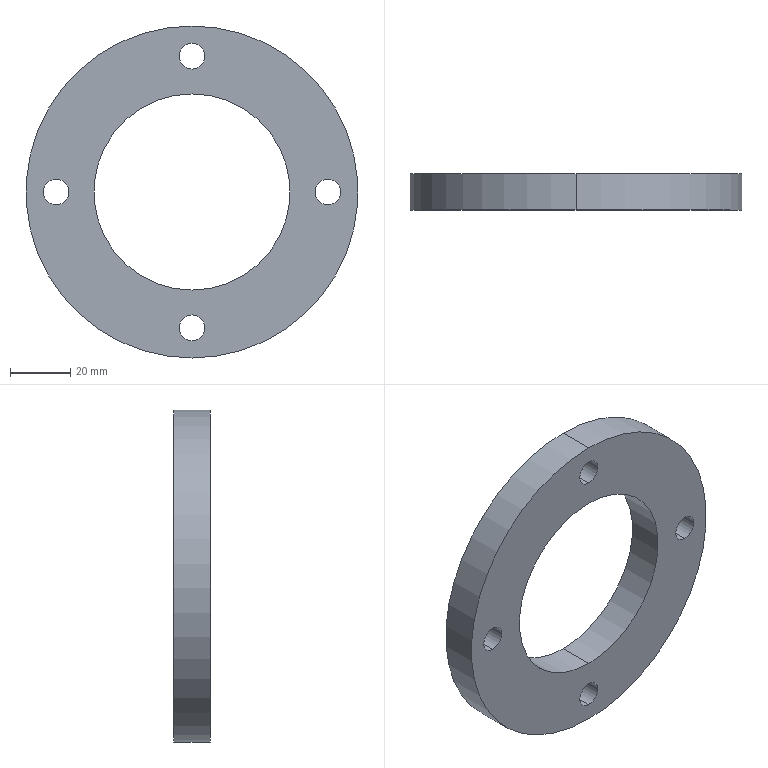Part | SolidWorks | features BaseBody 1 | 1 solid | 14 faces | box 110 x 12 x 110 mm | volume 71496 mm3 | cylinder 12 | plane 2 | commonest cylinder face diameters 8.5 x8 65 x2 110 x2
STEP:
#1=CARTESIAN_POINT('',(0.,12.,32.5));
#2=VERTEX_POINT('',#1);
#3=CARTESIAN_POINT('',(0.,12.,-32.5));
#4=VERTEX_POINT('',#3);
#5=CARTESIAN_POINT('',(0.,12.,0.));
#6=DIRECTION('',(0.,-1.,0.));
#7=DIRECTION('',(0.,0.,-1.));
#8=AXIS2_PLACEMENT_3D('',#5,#6,#7);
#9=CIRCLE('',#8,32.5);
#10=EDGE_CURVE('',#2,#4,#9,.T.);
#11=ORIENTED_EDGE('',*,*,#10,.F.);
#12=CARTESIAN_POINT('',(0.,0.,32.5));
#13=VERTEX_POINT('',#12);
#14=CARTESIAN_POINT('',(0.,12.,32.5));
#15=DIRECTION('',(0.,-1.,0.));
#16=VECTOR('',#15,1000.);
#17=LINE('',#14,#16);
#18=EDGE_CURVE('',#2,#13,#17,.T.);
#19=ORIENTED_EDGE('',*,*,#18,.T.);
#20=CARTESIAN_POINT('',(0.,0.,-32.5));
#21=VERTEX_POINT('',#20);
#22=CARTESIAN_POINT('',(0.,0.,0.));
#23=DIRECTION('',(0.,1.,0.));
#24=DIRECTION('',(0.,0.,-1.));
#25=AXIS2_PLACEMENT_3D('',#22,#23,#24);
#26=CIRCLE('',#25,32.5);
#27=EDGE_CURVE('',#21,#13,#26,.T.);
#28=ORIENTED_EDGE('',*,*,#27,.F.);
#29=CARTESIAN_POINT('',(0.,12.,-32.5));
#30=DIRECTION('',(0.,-1.,0.));
#31=VECTOR('',#30,1000.);
#32=LINE('',#29,#31);
#33=EDGE_CURVE('',#4,#21,#32,.T.);
#34=ORIENTED_EDGE('',*,*,#33,.F.);
#35=EDGE_LOOP('',(#11,#19,#28,#34));
#36=FACE_OUTER_BOUND('',#35,.T.);
#37=CARTESIAN_POINT('',(0.,12.,0.));
#38=DIRECTION('',(0.,-1.,0.));
#39=DIRECTION('',(0.,0.,-1.));
#40=AXIS2_PLACEMENT_3D('',#37,#38,#39);
#41=CYLINDRICAL_SURFACE('',#40,32.5);
#42=ADVANCED_FACE('',(#36),#41,.F.);
#43=CARTESIAN_POINT('',(0.,12.,55.));
#44=VERTEX_POINT('',#43);
#45=CARTESIAN_POINT('',(0.,12.,-55.));
#46=VERTEX_POINT('',#45);
#47=CARTESIAN_POINT('',(0.,12.,0.));
#48=DIRECTION('',(0.,1.,0.));
#49=DIRECTION('',(0.,0.,-1.));
#50=AXIS2_PLACEMENT_3D('',#47,#48,#49);
#51=CIRCLE('',#50,55.);
#52=EDGE_CURVE('',#44,#46,#51,.T.);
#53=ORIENTED_EDGE('',*,*,#52,.F.);
#54=CARTESIAN_POINT('',(0.,0.,55.));
#55=VERTEX_POINT('',#54);
#56=CARTESIAN_POINT('',(0.,12.,55.));
#57=DIRECTION('',(0.,-1.,0.));
#58=VECTOR('',#57,1000.);
#59=LINE('',#56,#58);
#60=EDGE_CURVE('',#44,#55,#59,.T.);
#61=ORIENTED_EDGE('',*,*,#60,.T.);
#62=CARTESIAN_POINT('',(0.,0.,-55.));
#63=VERTEX_POINT('',#62);
#64=CARTESIAN_POINT('',(0.,0.,0.));
#65=DIRECTION('',(0.,1.,0.));
#66=DIRECTION('',(0.,0.,-1.));
#67=AXIS2_PLACEMENT_3D('',#64,#65,#66);
#68=CIRCLE('',#67,55.);
#69=EDGE_CURVE('',#55,#63,#68,.T.);
#70=ORIENTED_EDGE('',*,*,#69,.T.);
#71=CARTESIAN_POINT('',(0.,12.,-55.));
#72=DIRECTION('',(0.,-1.,0.));
#73=VECTOR('',#72,1000.);
#74=LINE('',#71,#73);
#75=EDGE_CURVE('',#46,#63,#74,.T.);
#76=ORIENTED_EDGE('',*,*,#75,.F.);
#77=EDGE_LOOP('',(#53,#61,#70,#76));
#78=FACE_OUTER_BOUND('',#77,.T.);
#79=CARTESIAN_POINT('',(0.,12.,0.));
#80=DIRECTION('',(0.,-1.,0.));
#81=DIRECTION('',(0.,0.,-1.));
#82=AXIS2_PLACEMENT_3D('',#79,#80,#81);
#83=CYLINDRICAL_SURFACE('',#82,55.);
#84=ADVANCED_FACE('',(#78),#83,.T.);
#85=CARTESIAN_POINT('',(0.,0.,-49.25));
#86=VERTEX_POINT('',#85);
#87=CARTESIAN_POINT('',(0.,0.,-40.75));
#88=VERTEX_POINT('',#87);
#89=CARTESIAN_POINT('',(0.,0.,-45.));
#90=DIRECTION('',(0.,1.,0.));
#91=DIRECTION('',(0.,0.,1.));
#92=AXIS2_PLACEMENT_3D('',#89,#90,#91);
#93=CIRCLE('',#92,4.25);
#94=EDGE_CURVE('',#86,#88,#93,.T.);
#95=ORIENTED_EDGE('',*,*,#94,.F.);
#96=CARTESIAN_POINT('',(0.,12.,-49.25));
#97=VERTEX_POINT('',#96);
#98=CARTESIAN_POINT('',(0.,12.,-49.25));
#99=DIRECTION('',(0.,1.,0.));
#100=VECTOR('',#99,1000.);
#101=LINE('',#98,#100);
#102=EDGE_CURVE('',#86,#97,#101,.T.);
#103=ORIENTED_EDGE('',*,*,#102,.T.);
#104=CARTESIAN_POINT('',(0.,12.,-40.75));
#105=VERTEX_POINT('',#104);
#106=CARTESIAN_POINT('',(0.,12.,-45.));
#107=DIRECTION('',(0.,-1.,0.));
#108=DIRECTION('',(0.,0.,1.));
#109=AXIS2_PLACEMENT_3D('',#106,#107,#108);
#110=CIRCLE('',#109,4.25);
#111=EDGE_CURVE('',#105,#97,#110,.T.);
#112=ORIENTED_EDGE('',*,*,#111,.F.);
#113=CARTESIAN_POINT('',(0.,12.,-40.75));
#114=DIRECTION('',(0.,1.,0.));
#115=VECTOR('',#114,1000.);
#116=LINE('',#113,#115);
#117=EDGE_CURVE('',#88,#105,#116,.T.);
#118=ORIENTED_EDGE('',*,*,#117,.F.);
#119=EDGE_LOOP('',(#95,#103,#112,#118));
#120=FACE_OUTER_BOUND('',#119,.T.);
#121=CARTESIAN_POINT('',(0.,12.,-45.));
#122=DIRECTION('',(0.,1.,0.));
#123=DIRECTION('',(0.,0.,1.));
#124=AXIS2_PLACEMENT_3D('',#121,#122,#123);
#125=CYLINDRICAL_SURFACE('',#124,4.25);
#126=ADVANCED_FACE('',(#120),#125,.F.);
#127=CARTESIAN_POINT('',(-45.,0.,-4.25));
#128=VERTEX_POINT('',#127);
#129=CARTESIAN_POINT('',(-45.,0.,4.25));
#130=VERTEX_POINT('',#129);
#131=CARTESIAN_POINT('',(-45.,0.,0.));
#132=DIRECTION('',(0.,1.,0.));
#133=DIRECTION('',(0.,0.,1.));
#134=AXIS2_PLACEMENT_3D('',#131,#132,#133);
#135=CIRCLE('',#134,4.25);
#136=EDGE_CURVE('',#128,#130,#135,.T.);
#137=ORIENTED_EDGE('',*,*,#136,.F.);
#138=CARTESIAN_POINT('',(-45.,12.,-4.25));
#139=VERTEX_POINT('',#138);
#140=CARTESIAN_POINT('',(-45.,12.,-4.25));
#141=DIRECTION('',(0.,1.,0.));
#142=VECTOR('',#141,1000.);
#143=LINE('',#140,#142);
#144=EDGE_CURVE('',#128,#139,#143,.T.);
#145=ORIENTED_EDGE('',*,*,#144,.T.);
#146=CARTESIAN_POINT('',(-45.,12.,4.25));
#147=VERTEX_POINT('',#146);
#148=CARTESIAN_POINT('',(-45.,12.,0.));
#149=DIRECTION('',(0.,-1.,0.));
#150=DIRECTION('',(0.,0.,1.));
#151=AXIS2_PLACEMENT_3D('',#148,#149,#150);
#152=CIRCLE('',#151,4.25);
#153=EDGE_CURVE('',#147,#139,#152,.T.);
#154=ORIENTED_EDGE('',*,*,#153,.F.);
#155=CARTESIAN_POINT('',(-45.,12.,4.25));
#156=DIRECTION('',(0.,1.,0.));
#157=VECTOR('',#156,1000.);
#158=LINE('',#155,#157);
#159=EDGE_CURVE('',#130,#147,#158,.T.);
#160=ORIENTED_EDGE('',*,*,#159,.F.);
#161=EDGE_LOOP('',(#137,#145,#154,#160));
#162=FACE_OUTER_BOUND('',#161,.T.);
#163=CARTESIAN_POINT('',(-45.,12.,0.));
#164=DIRECTION('',(0.,1.,0.));
#165=DIRECTION('',(0.,0.,1.));
#166=AXIS2_PLACEMENT_3D('',#163,#164,#165);
#167=CYLINDRICAL_SURFACE('',#166,4.25);
#168=ADVANCED_FACE('',(#162),#167,.F.);
#169=CARTESIAN_POINT('',(0.,0.,40.75));
#170=VERTEX_POINT('',#169);
#171=CARTESIAN_POINT('',(0.,0.,49.25));
#172=VERTEX_POINT('',#171);
#173=CARTESIAN_POINT('',(0.,0.,45.));
#174=DIRECTION('',(0.,1.,0.));
#175=DIRECTION('',(0.,0.,1.));
#176=AXIS2_PLACEMENT_3D('',#173,#174,#175);
#177=CIRCLE('',#176,4.25);
#178=EDGE_CURVE('',#170,#172,#177,.T.);
#179=ORIENTED_EDGE('',*,*,#178,.F.);
#180=CARTESIAN_POINT('',(0.,12.,40.75));
#181=VERTEX_POINT('',#180);
#182=CARTESIAN_POINT('',(0.,12.,40.75));
#183=DIRECTION('',(0.,1.,0.));
#184=VECTOR('',#183,1000.);
#185=LINE('',#182,#184);
#186=EDGE_CURVE('',#170,#181,#185,.T.);
#187=ORIENTED_EDGE('',*,*,#186,.T.);
#188=CARTESIAN_POINT('',(0.,12.,49.25));
#189=VERTEX_POINT('',#188);
#190=CARTESIAN_POINT('',(0.,12.,45.));
#191=DIRECTION('',(0.,-1.,0.));
#192=DIRECTION('',(0.,0.,1.));
#193=AXIS2_PLACEMENT_3D('',#190,#191,#192);
#194=CIRCLE('',#193,4.25);
#195=EDGE_CURVE('',#189,#181,#194,.T.);
#196=ORIENTED_EDGE('',*,*,#195,.F.);
#197=CARTESIAN_POINT('',(0.,12.,49.25));
#198=DIRECTION('',(0.,1.,0.));
#199=VECTOR('',#198,1000.);
#200=LINE('',#197,#199);
#201=EDGE_CURVE('',#172,#189,#200,.T.);
#202=ORIENTED_EDGE('',*,*,#201,.F.);
#203=EDGE_LOOP('',(#179,#187,#196,#202));
#204=FACE_OUTER_BOUND('',#203,.T.);
#205=CARTESIAN_POINT('',(0.,12.,45.));
#206=DIRECTION('',(0.,1.,0.));
#207=DIRECTION('',(0.,0.,1.));
#208=AXIS2_PLACEMENT_3D('',#205,#206,#207);
#209=CYLINDRICAL_SURFACE('',#208,4.25);
#210=ADVANCED_FACE('',(#204),#209,.F.);
#211=CARTESIAN_POINT('',(45.,0.,-4.25));
#212=VERTEX_POINT('',#211);
#213=CARTESIAN_POINT('',(45.,0.,4.25));
#214=VERTEX_POINT('',#213);
#215=CARTESIAN_POINT('',(45.,0.,0.));
#216=DIRECTION('',(0.,1.,0.));
#217=DIRECTION('',(0.,0.,1.));
#218=AXIS2_PLACEMENT_3D('',#215,#216,#217);
#219=CIRCLE('',#218,4.25);
#220=EDGE_CURVE('',#212,#214,#219,.T.);
#221=ORIENTED_EDGE('',*,*,#220,.F.);
#222=CARTESIAN_POINT('',(45.,12.,-4.25));
#223=VERTEX_POINT('',#222);
#224=CARTESIAN_POINT('',(45.,12.,-4.25));
#225=DIRECTION('',(0.,1.,0.));
#226=VECTOR('',#225,1000.);
#227=LINE('',#224,#226);
#228=EDGE_CURVE('',#212,#223,#227,.T.);
#229=ORIENTED_EDGE('',*,*,#228,.T.);
#230=CARTESIAN_POINT('',(45.,12.,4.25));
#231=VERTEX_POINT('',#230);
#232=CARTESIAN_POINT('',(45.,12.,0.));
#233=DIRECTION('',(0.,-1.,0.));
#234=DIRECTION('',(0.,0.,1.));
#235=AXIS2_PLACEMENT_3D('',#232,#233,#234);
#236=CIRCLE('',#235,4.25);
#237=EDGE_CURVE('',#231,#223,#236,.T.);
#238=ORIENTED_EDGE('',*,*,#237,.F.);
#239=CARTESIAN_POINT('',(45.,12.,4.25));
#240=DIRECTION('',(0.,1.,0.));
#241=VECTOR('',#240,1000.);
#242=LINE('',#239,#241);
#243=EDGE_CURVE('',#214,#231,#242,.T.);
#244=ORIENTED_EDGE('',*,*,#243,.F.);
#245=EDGE_LOOP('',(#221,#229,#238,#244));
#246=FACE_OUTER_BOUND('',#245,.T.);
#247=CARTESIAN_POINT('',(45.,12.,0.));
#248=DIRECTION('',(0.,1.,0.));
#249=DIRECTION('',(0.,0.,1.));
#250=AXIS2_PLACEMENT_3D('',#247,#248,#249);
#251=CYLINDRICAL_SURFACE('',#250,4.25);
#252=ADVANCED_FACE('',(#246),#251,.F.);
#253=CARTESIAN_POINT('',(0.,12.,0.));
#254=DIRECTION('',(0.,-1.,0.));
#255=DIRECTION('',(0.,0.,-1.));
#256=AXIS2_PLACEMENT_3D('',#253,#254,#255);
#257=CIRCLE('',#256,32.5);
#258=EDGE_CURVE('',#4,#2,#257,.T.);
#259=ORIENTED_EDGE('',*,*,#258,.T.);
#260=ORIENTED_EDGE('',*,*,#10,.T.);
#261=EDGE_LOOP('',(#259,#260));
#262=FACE_BOUND('',#261,.T.);
#263=CARTESIAN_POINT('',(0.,12.,0.));
#264=DIRECTION('',(0.,1.,0.));
#265=DIRECTION('',(0.,0.,-1.));
#266=AXIS2_PLACEMENT_3D('',#263,#264,#265);
#267=CIRCLE('',#266,55.);
#268=EDGE_CURVE('',#46,#44,#267,.T.);
#269=ORIENTED_EDGE('',*,*,#268,.T.);
#270=ORIENTED_EDGE('',*,*,#52,.T.);
#271=EDGE_LOOP('',(#269,#270));
#272=FACE_OUTER_BOUND('',#271,.T.);
#273=ORIENTED_EDGE('',*,*,#111,.T.);
#274=CARTESIAN_POINT('',(0.,12.,-45.));
#275=DIRECTION('',(0.,-1.,0.));
#276=DIRECTION('',(0.,0.,1.));
#277=AXIS2_PLACEMENT_3D('',#274,#275,#276);
#278=CIRCLE('',#277,4.25);
#279=EDGE_CURVE('',#97,#105,#278,.T.);
#280=ORIENTED_EDGE('',*,*,#279,.T.);
#281=EDGE_LOOP('',(#273,#280));
#282=FACE_BOUND('',#281,.T.);
#283=ORIENTED_EDGE('',*,*,#153,.T.);
#284=CARTESIAN_POINT('',(-45.,12.,0.));
#285=DIRECTION('',(0.,-1.,0.));
#286=DIRECTION('',(0.,0.,1.));
#287=AXIS2_PLACEMENT_3D('',#284,#285,#286);
#288=CIRCLE('',#287,4.25);
#289=EDGE_CURVE('',#139,#147,#288,.T.);
#290=ORIENTED_EDGE('',*,*,#289,.T.);
#291=EDGE_LOOP('',(#283,#290));
#292=FACE_BOUND('',#291,.T.);
#293=ORIENTED_EDGE('',*,*,#195,.T.);
#294=CARTESIAN_POINT('',(0.,12.,45.));
#295=DIRECTION('',(0.,-1.,0.));
#296=DIRECTION('',(0.,0.,1.));
#297=AXIS2_PLACEMENT_3D('',#294,#295,#296);
#298=CIRCLE('',#297,4.25);
#299=EDGE_CURVE('',#181,#189,#298,.T.);
#300=ORIENTED_EDGE('',*,*,#299,.T.);
#301=EDGE_LOOP('',(#293,#300));
#302=FACE_BOUND('',#301,.T.);
#303=ORIENTED_EDGE('',*,*,#237,.T.);
#304=CARTESIAN_POINT('',(45.,12.,0.));
#305=DIRECTION('',(0.,-1.,0.));
#306=DIRECTION('',(0.,0.,1.));
#307=AXIS2_PLACEMENT_3D('',#304,#305,#306);
#308=CIRCLE('',#307,4.25);
#309=EDGE_CURVE('',#223,#231,#308,.T.);
#310=ORIENTED_EDGE('',*,*,#309,.T.);
#311=EDGE_LOOP('',(#303,#310));
#312=FACE_BOUND('',#311,.T.);
#313=CARTESIAN_POINT('',(0.,12.,0.));
#314=DIRECTION('',(0.,1.,0.));
#315=DIRECTION('',(0.,0.,1.));
#316=AXIS2_PLACEMENT_3D('',#313,#314,#315);
#317=PLANE('',#316);
#318=ADVANCED_FACE('',(#262,#272,#282,#292,#302,#312),#317,.T.);
#319=ORIENTED_EDGE('',*,*,#18,.F.);
#320=ORIENTED_EDGE('',*,*,#258,.F.);
#321=ORIENTED_EDGE('',*,*,#33,.T.);
#322=CARTESIAN_POINT('',(0.,0.,0.));
#323=DIRECTION('',(0.,1.,0.));
#324=DIRECTION('',(0.,0.,-1.));
#325=AXIS2_PLACEMENT_3D('',#322,#323,#324);
#326=CIRCLE('',#325,32.5);
#327=EDGE_CURVE('',#13,#21,#326,.T.);
#328=ORIENTED_EDGE('',*,*,#327,.F.);
#329=EDGE_LOOP('',(#319,#320,#321,#328));
#330=FACE_OUTER_BOUND('',#329,.T.);
#331=CARTESIAN_POINT('',(0.,12.,0.));
#332=DIRECTION('',(0.,-1.,0.));
#333=DIRECTION('',(0.,0.,-1.));
#334=AXIS2_PLACEMENT_3D('',#331,#332,#333);
#335=CYLINDRICAL_SURFACE('',#334,32.5);
#336=ADVANCED_FACE('',(#330),#335,.F.);
#337=ORIENTED_EDGE('',*,*,#60,.F.);
#338=ORIENTED_EDGE('',*,*,#268,.F.);
#339=ORIENTED_EDGE('',*,*,#75,.T.);
#340=CARTESIAN_POINT('',(0.,0.,0.));
#341=DIRECTION('',(0.,1.,0.));
#342=DIRECTION('',(0.,0.,-1.));
#343=AXIS2_PLACEMENT_3D('',#340,#341,#342);
#344=CIRCLE('',#343,55.);
#345=EDGE_CURVE('',#63,#55,#344,.T.);
#346=ORIENTED_EDGE('',*,*,#345,.T.);
#347=EDGE_LOOP('',(#337,#338,#339,#346));
#348=FACE_OUTER_BOUND('',#347,.T.);
#349=CARTESIAN_POINT('',(0.,12.,0.));
#350=DIRECTION('',(0.,-1.,0.));
#351=DIRECTION('',(0.,0.,-1.));
#352=AXIS2_PLACEMENT_3D('',#349,#350,#351);
#353=CYLINDRICAL_SURFACE('',#352,55.);
#354=ADVANCED_FACE('',(#348),#353,.T.);
#355=ORIENTED_EDGE('',*,*,#102,.F.);
#356=CARTESIAN_POINT('',(0.,0.,-45.));
#357=DIRECTION('',(0.,1.,0.));
#358=DIRECTION('',(0.,0.,1.));
#359=AXIS2_PLACEMENT_3D('',#356,#357,#358);
#360=CIRCLE('',#359,4.25);
#361=EDGE_CURVE('',#88,#86,#360,.T.);
#362=ORIENTED_EDGE('',*,*,#361,.F.);
#363=ORIENTED_EDGE('',*,*,#117,.T.);
#364=ORIENTED_EDGE('',*,*,#279,.F.);
#365=EDGE_LOOP('',(#355,#362,#363,#364));
#366=FACE_OUTER_BOUND('',#365,.T.);
#367=CARTESIAN_POINT('',(0.,12.,-45.));
#368=DIRECTION('',(0.,1.,0.));
#369=DIRECTION('',(0.,0.,1.));
#370=AXIS2_PLACEMENT_3D('',#367,#368,#369);
#371=CYLINDRICAL_SURFACE('',#370,4.25);
#372=ADVANCED_FACE('',(#366),#371,.F.);
#373=ORIENTED_EDGE('',*,*,#144,.F.);
#374=CARTESIAN_POINT('',(-45.,0.,0.));
#375=DIRECTION('',(0.,1.,0.));
#376=DIRECTION('',(0.,0.,1.));
#377=AXIS2_PLACEMENT_3D('',#374,#375,#376);
#378=CIRCLE('',#377,4.25);
#379=EDGE_CURVE('',#130,#128,#378,.T.);
#380=ORIENTED_EDGE('',*,*,#379,.F.);
#381=ORIENTED_EDGE('',*,*,#159,.T.);
#382=ORIENTED_EDGE('',*,*,#289,.F.);
#383=EDGE_LOOP('',(#373,#380,#381,#382));
#384=FACE_OUTER_BOUND('',#383,.T.);
#385=CARTESIAN_POINT('',(-45.,12.,0.));
#386=DIRECTION('',(0.,1.,0.));
#387=DIRECTION('',(0.,0.,1.));
#388=AXIS2_PLACEMENT_3D('',#385,#386,#387);
#389=CYLINDRICAL_SURFACE('',#388,4.25);
#390=ADVANCED_FACE('',(#384),#389,.F.);
#391=ORIENTED_EDGE('',*,*,#186,.F.);
#392=CARTESIAN_POINT('',(0.,0.,45.));
#393=DIRECTION('',(0.,1.,0.));
#394=DIRECTION('',(0.,0.,1.));
#395=AXIS2_PLACEMENT_3D('',#392,#393,#394);
#396=CIRCLE('',#395,4.25);
#397=EDGE_CURVE('',#172,#170,#396,.T.);
#398=ORIENTED_EDGE('',*,*,#397,.F.);
#399=ORIENTED_EDGE('',*,*,#201,.T.);
#400=ORIENTED_EDGE('',*,*,#299,.F.);
#401=EDGE_LOOP('',(#391,#398,#399,#400));
#402=FACE_OUTER_BOUND('',#401,.T.);
#403=CARTESIAN_POINT('',(0.,12.,45.));
#404=DIRECTION('',(0.,1.,0.));
#405=DIRECTION('',(0.,0.,1.));
#406=AXIS2_PLACEMENT_3D('',#403,#404,#405);
#407=CYLINDRICAL_SURFACE('',#406,4.25);
#408=ADVANCED_FACE('',(#402),#407,.F.);
#409=ORIENTED_EDGE('',*,*,#228,.F.);
#410=CARTESIAN_POINT('',(45.,0.,0.));
#411=DIRECTION('',(0.,1.,0.));
#412=DIRECTION('',(0.,0.,1.));
#413=AXIS2_PLACEMENT_3D('',#410,#411,#412);
#414=CIRCLE('',#413,4.25);
#415=EDGE_CURVE('',#214,#212,#414,.T.);
#416=ORIENTED_EDGE('',*,*,#415,.F.);
#417=ORIENTED_EDGE('',*,*,#243,.T.);
#418=ORIENTED_EDGE('',*,*,#309,.F.);
#419=EDGE_LOOP('',(#409,#416,#417,#418));
#420=FACE_OUTER_BOUND('',#419,.T.);
#421=CARTESIAN_POINT('',(45.,12.,0.));
#422=DIRECTION('',(0.,1.,0.));
#423=DIRECTION('',(0.,0.,1.));
#424=AXIS2_PLACEMENT_3D('',#421,#422,#423);
#425=CYLINDRICAL_SURFACE('',#424,4.25);
#426=ADVANCED_FACE('',(#420),#425,.F.);
#427=ORIENTED_EDGE('',*,*,#27,.T.);
#428=ORIENTED_EDGE('',*,*,#327,.T.);
#429=EDGE_LOOP('',(#427,#428));
#430=FACE_BOUND('',#429,.T.);
#431=ORIENTED_EDGE('',*,*,#345,.F.);
#432=ORIENTED_EDGE('',*,*,#69,.F.);
#433=EDGE_LOOP('',(#431,#432));
#434=FACE_OUTER_BOUND('',#433,.T.);
#435=ORIENTED_EDGE('',*,*,#361,.T.);
#436=ORIENTED_EDGE('',*,*,#94,.T.);
#437=EDGE_LOOP('',(#435,#436));
#438=FACE_BOUND('',#437,.T.);
#439=ORIENTED_EDGE('',*,*,#379,.T.);
#440=ORIENTED_EDGE('',*,*,#136,.T.);
#441=EDGE_LOOP('',(#439,#440));
#442=FACE_BOUND('',#441,.T.);
#443=ORIENTED_EDGE('',*,*,#397,.T.);
#444=ORIENTED_EDGE('',*,*,#178,.T.);
#445=EDGE_LOOP('',(#443,#444));
#446=FACE_BOUND('',#445,.T.);
#447=ORIENTED_EDGE('',*,*,#415,.T.);
#448=ORIENTED_EDGE('',*,*,#220,.T.);
#449=EDGE_LOOP('',(#447,#448));
#450=FACE_BOUND('',#449,.T.);
#451=CARTESIAN_POINT('',(0.,0.,0.));
#452=DIRECTION('',(0.,1.,0.));
#453=DIRECTION('',(0.,0.,1.));
#454=AXIS2_PLACEMENT_3D('',#451,#452,#453);
#455=PLANE('',#454);
#456=ADVANCED_FACE('',(#430,#434,#438,#442,#446,#450),#455,.F.);
#457=CLOSED_SHELL('',(#42,#84,#126,#168,#210,#252,#318,#336,#354,#372,#390,#408,#426,#456));
#458=MANIFOLD_SOLID_BREP('',#457);
#459=CARTESIAN_POINT('',(0.,0.,0.));
#460=DIRECTION('',(0.,0.,1.));
#461=DIRECTION('',(1.,0.,0.));
#462=AXIS2_PLACEMENT_3D('',#459,#460,#461);
#463=(LENGTH_UNIT()NAMED_UNIT(*)SI_UNIT(.MILLI.,.METRE.));
#464=UNCERTAINTY_MEASURE_WITH_UNIT(LENGTH_MEASURE(0.00001),#463,'','');
#465=(NAMED_UNIT(*)PLANE_ANGLE_UNIT()SI_UNIT($,.RADIAN.));
#466=(NAMED_UNIT(*)SI_UNIT($,.STERADIAN.)SOLID_ANGLE_UNIT());
#467=(GEOMETRIC_REPRESENTATION_CONTEXT(3)GLOBAL_UNCERTAINTY_ASSIGNED_CONTEXT((#464))GLOBAL_UNIT_ASSIGNED_CONTEXT((#463,#465,#466))REPRESENTATION_CONTEXT('',''));
#468=ADVANCED_BREP_SHAPE_REPRESENTATION('',(#458,#462),#467);